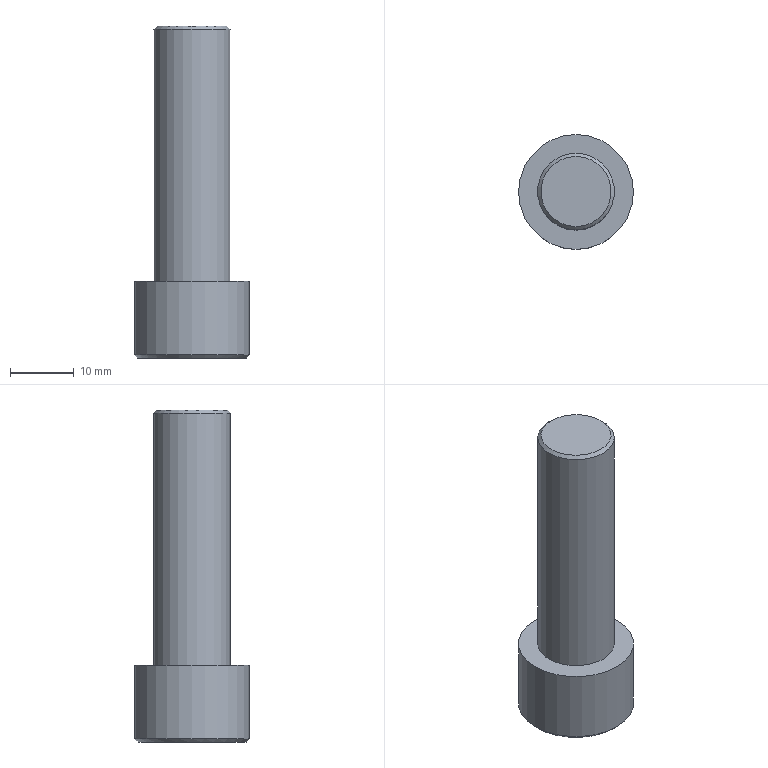Part | STEP file | 1_id1798_x_t | 1 solid | 21 faces | box 18 x 18 x 52 mm | volume 7011 mm3 | plane 15 | cone 4 | cylinder 2 | commonest cylinder face diameters 12 x1 18 x1
STEP:
#1=CARTESIAN_POINT('',(2147.435,399.726,-28.5));
#2=VERTEX_POINT('',#1);
#3=CARTESIAN_POINT('',(2147.435,405.5,-27.5));
#4=VERTEX_POINT('',#3);
#5=CARTESIAN_POINT('',(2147.435,402.613,-28.));
#6=DIRECTION('',(0.,0.9853,0.1707));
#7=VECTOR('',#6,1.);
#8=LINE('',#5,#7);
#9=EDGE_CURVE('',#2,#4,#8,.T.);
#10=ORIENTED_EDGE('',*,*,#9,.T.);
#11=CARTESIAN_POINT('',(2147.435,411.274,-28.5));
#12=VERTEX_POINT('',#11);
#13=CARTESIAN_POINT('',(2147.435,408.387,-28.));
#14=DIRECTION('',(0.,0.9853,-0.1707));
#15=VECTOR('',#14,1.);
#16=LINE('',#13,#15);
#17=EDGE_CURVE('',#4,#12,#16,.T.);
#18=ORIENTED_EDGE('',*,*,#17,.T.);
#19=CARTESIAN_POINT('',(2150.322,410.5,-28.5));
#20=VERTEX_POINT('',#19);
#21=CARTESIAN_POINT('',(2147.435,405.5,-28.5));
#22=DIRECTION('',(0.,0.,-1.));
#23=DIRECTION('',(0.,1.,0.));
#24=AXIS2_PLACEMENT_3D('',#21,#22,#23);
#25=CIRCLE('',#24,5.774);
#26=EDGE_CURVE('',#12,#20,#25,.T.);
#27=ORIENTED_EDGE('',*,*,#26,.T.);
#28=CARTESIAN_POINT('',(2153.209,405.5,-28.5));
#29=VERTEX_POINT('',#28);
#30=CARTESIAN_POINT('',(2147.435,405.5,-28.5));
#31=DIRECTION('',(0.,0.,-1.));
#32=DIRECTION('',(0.,1.,0.));
#33=AXIS2_PLACEMENT_3D('',#30,#31,#32);
#34=CIRCLE('',#33,5.774);
#35=EDGE_CURVE('',#20,#29,#34,.T.);
#36=ORIENTED_EDGE('',*,*,#35,.T.);
#37=CARTESIAN_POINT('',(2150.322,400.5,-28.5));
#38=VERTEX_POINT('',#37);
#39=CARTESIAN_POINT('',(2147.435,405.5,-28.5));
#40=DIRECTION('',(0.,0.,-1.));
#41=DIRECTION('',(0.,1.,0.));
#42=AXIS2_PLACEMENT_3D('',#39,#40,#41);
#43=CIRCLE('',#42,5.774);
#44=EDGE_CURVE('',#29,#38,#43,.T.);
#45=ORIENTED_EDGE('',*,*,#44,.T.);
#46=CARTESIAN_POINT('',(2147.435,405.5,-28.5));
#47=DIRECTION('',(0.,0.,-1.));
#48=DIRECTION('',(0.,1.,0.));
#49=AXIS2_PLACEMENT_3D('',#46,#47,#48);
#50=CIRCLE('',#49,5.774);
#51=EDGE_CURVE('',#38,#2,#50,.T.);
#52=ORIENTED_EDGE('',*,*,#51,.T.);
#53=EDGE_LOOP('',(#10,#18,#27,#36,#45,#52));
#54=FACE_OUTER_BOUND('',#53,.T.);
#55=CARTESIAN_POINT('',(2147.435,405.5,-28.));
#56=DIRECTION('',(0.,0.,-1.));
#57=DIRECTION('',(0.,-1.,0.));
#58=AXIS2_PLACEMENT_3D('',#55,#56,#57);
#59=CONICAL_SURFACE('',#58,2.887,80.174);
#60=ADVANCED_FACE('',(#54),#59,.F.);
#61=CARTESIAN_POINT('',(2147.435,399.5,17.));
#62=VERTEX_POINT('',#61);
#63=CARTESIAN_POINT('',(2147.435,405.5,17.));
#64=DIRECTION('',(0.,0.,1.));
#65=DIRECTION('',(0.,-1.,0.));
#66=AXIS2_PLACEMENT_3D('',#63,#64,#65);
#67=CIRCLE('',#66,6.);
#68=EDGE_CURVE('',#62,#62,#67,.T.);
#69=ORIENTED_EDGE('',*,*,#68,.T.);
#70=EDGE_LOOP('',(#69));
#71=FACE_BOUND('',#70,.T.);
#72=CARTESIAN_POINT('',(2147.435,400.,17.5));
#73=VERTEX_POINT('',#72);
#74=CARTESIAN_POINT('',(2147.435,405.5,17.5));
#75=DIRECTION('',(0.,0.,-1.));
#76=DIRECTION('',(0.,-1.,0.));
#77=AXIS2_PLACEMENT_3D('',#74,#75,#76);
#78=CIRCLE('',#77,5.5);
#79=EDGE_CURVE('',#73,#73,#78,.T.);
#80=ORIENTED_EDGE('',*,*,#79,.T.);
#81=EDGE_LOOP('',(#80));
#82=FACE_BOUND('',#81,.T.);
#83=CARTESIAN_POINT('',(2147.435,405.5,17.5));
#84=DIRECTION('',(0.,0.,-1.));
#85=DIRECTION('',(0.,1.,0.));
#86=AXIS2_PLACEMENT_3D('',#83,#84,#85);
#87=CONICAL_SURFACE('',#86,5.5,45.);
#88=ADVANCED_FACE('',(#71,#82),#87,.T.);
#89=ORIENTED_EDGE('',*,*,#68,.F.);
#90=EDGE_LOOP('',(#89));
#91=FACE_BOUND('',#90,.T.);
#92=CARTESIAN_POINT('',(2147.435,411.5,-22.5));
#93=VERTEX_POINT('',#92);
#94=CARTESIAN_POINT('',(2147.435,405.5,-22.5));
#95=DIRECTION('',(0.,0.,-1.));
#96=DIRECTION('',(0.,1.,0.));
#97=AXIS2_PLACEMENT_3D('',#94,#95,#96);
#98=CIRCLE('',#97,6.);
#99=EDGE_CURVE('',#93,#93,#98,.T.);
#100=ORIENTED_EDGE('',*,*,#99,.F.);
#101=EDGE_LOOP('',(#100));
#102=FACE_BOUND('',#101,.T.);
#103=CARTESIAN_POINT('',(2147.435,405.5,-2.5));
#104=DIRECTION('',(0.,0.,1.));
#105=DIRECTION('',(0.,-1.,0.));
#106=AXIS2_PLACEMENT_3D('',#103,#104,#105);
#107=CYLINDRICAL_SURFACE('',#106,6.);
#108=ADVANCED_FACE('',(#91,#102),#107,.T.);
#109=ORIENTED_EDGE('',*,*,#79,.F.);
#110=EDGE_LOOP('',(#109));
#111=FACE_OUTER_BOUND('',#110,.T.);
#112=CARTESIAN_POINT('',(2147.435,405.5,17.5));
#113=DIRECTION('',(0.,0.,1.));
#114=DIRECTION('',(0.,-1.,0.));
#115=AXIS2_PLACEMENT_3D('',#112,#113,#114);
#116=PLANE('',#115);
#117=ADVANCED_FACE('',(#111),#116,.T.);
#118=CARTESIAN_POINT('',(2147.435,396.5,-34.));
#119=VERTEX_POINT('',#118);
#120=CARTESIAN_POINT('',(2147.435,405.5,-34.));
#121=DIRECTION('',(0.,0.,-1.));
#122=DIRECTION('',(0.,-1.,0.));
#123=AXIS2_PLACEMENT_3D('',#120,#121,#122);
#124=CIRCLE('',#123,9.);
#125=EDGE_CURVE('',#119,#119,#124,.T.);
#126=ORIENTED_EDGE('',*,*,#125,.T.);
#127=EDGE_LOOP('',(#126));
#128=FACE_BOUND('',#127,.T.);
#129=CARTESIAN_POINT('',(2147.435,397.,-34.5));
#130=VERTEX_POINT('',#129);
#131=CARTESIAN_POINT('',(2147.435,405.5,-34.5));
#132=DIRECTION('',(0.,0.,1.));
#133=DIRECTION('',(0.,-1.,0.));
#134=AXIS2_PLACEMENT_3D('',#131,#132,#133);
#135=CIRCLE('',#134,8.5);
#136=EDGE_CURVE('',#130,#130,#135,.T.);
#137=ORIENTED_EDGE('',*,*,#136,.T.);
#138=EDGE_LOOP('',(#137));
#139=FACE_BOUND('',#138,.T.);
#140=CARTESIAN_POINT('',(2147.435,405.5,-34.5));
#141=DIRECTION('',(0.,0.,1.));
#142=DIRECTION('',(0.,1.,0.));
#143=AXIS2_PLACEMENT_3D('',#140,#141,#142);
#144=CONICAL_SURFACE('',#143,8.5,45.);
#145=ADVANCED_FACE('',(#128,#139),#144,.T.);
#146=CARTESIAN_POINT('',(2147.435,414.5,-22.5));
#147=VERTEX_POINT('',#146);
#148=CARTESIAN_POINT('',(2147.435,405.5,-22.5));
#149=DIRECTION('',(0.,0.,1.));
#150=DIRECTION('',(0.,1.,0.));
#151=AXIS2_PLACEMENT_3D('',#148,#149,#150);
#152=CIRCLE('',#151,9.);
#153=EDGE_CURVE('',#147,#147,#152,.T.);
#154=ORIENTED_EDGE('',*,*,#153,.F.);
#155=EDGE_LOOP('',(#154));
#156=FACE_BOUND('',#155,.T.);
#157=ORIENTED_EDGE('',*,*,#125,.F.);
#158=EDGE_LOOP('',(#157));
#159=FACE_BOUND('',#158,.T.);
#160=CARTESIAN_POINT('',(2147.435,405.5,-28.5));
#161=DIRECTION('',(0.,0.,1.));
#162=DIRECTION('',(0.,-1.,0.));
#163=AXIS2_PLACEMENT_3D('',#160,#161,#162);
#164=CYLINDRICAL_SURFACE('',#163,9.);
#165=ADVANCED_FACE('',(#156,#159),#164,.T.);
#166=CARTESIAN_POINT('',(2153.209,405.5,-34.5));
#167=VERTEX_POINT('',#166);
#168=CARTESIAN_POINT('',(2150.322,410.5,-34.5));
#169=VERTEX_POINT('',#168);
#170=CARTESIAN_POINT('',(2151.765,408.,-34.5));
#171=DIRECTION('',(-0.5,0.866,0.));
#172=VECTOR('',#171,1.);
#173=LINE('',#170,#172);
#174=EDGE_CURVE('',#167,#169,#173,.T.);
#175=ORIENTED_EDGE('',*,*,#174,.T.);
#176=CARTESIAN_POINT('',(2144.548,410.5,-34.5));
#177=VERTEX_POINT('',#176);
#178=CARTESIAN_POINT('',(2147.435,410.5,-34.5));
#179=DIRECTION('',(-1.,0.,0.));
#180=VECTOR('',#179,1.);
#181=LINE('',#178,#180);
#182=EDGE_CURVE('',#169,#177,#181,.T.);
#183=ORIENTED_EDGE('',*,*,#182,.T.);
#184=CARTESIAN_POINT('',(2141.662,405.5,-34.5));
#185=VERTEX_POINT('',#184);
#186=CARTESIAN_POINT('',(2143.105,408.,-34.5));
#187=DIRECTION('',(-0.5,-0.866,0.));
#188=VECTOR('',#187,1.);
#189=LINE('',#186,#188);
#190=EDGE_CURVE('',#177,#185,#189,.T.);
#191=ORIENTED_EDGE('',*,*,#190,.T.);
#192=CARTESIAN_POINT('',(2144.548,400.5,-34.5));
#193=VERTEX_POINT('',#192);
#194=CARTESIAN_POINT('',(2143.105,403.,-34.5));
#195=DIRECTION('',(0.5,-0.866,0.));
#196=VECTOR('',#195,1.);
#197=LINE('',#194,#196);
#198=EDGE_CURVE('',#185,#193,#197,.T.);
#199=ORIENTED_EDGE('',*,*,#198,.T.);
#200=CARTESIAN_POINT('',(2150.322,400.5,-34.5));
#201=VERTEX_POINT('',#200);
#202=CARTESIAN_POINT('',(2147.435,400.5,-34.5));
#203=DIRECTION('',(1.,0.,0.));
#204=VECTOR('',#203,1.);
#205=LINE('',#202,#204);
#206=EDGE_CURVE('',#193,#201,#205,.T.);
#207=ORIENTED_EDGE('',*,*,#206,.T.);
#208=CARTESIAN_POINT('',(2151.765,403.,-34.5));
#209=DIRECTION('',(0.5,0.866,0.));
#210=VECTOR('',#209,1.);
#211=LINE('',#208,#210);
#212=EDGE_CURVE('',#201,#167,#211,.T.);
#213=ORIENTED_EDGE('',*,*,#212,.T.);
#214=EDGE_LOOP('',(#175,#183,#191,#199,#207,#213));
#215=FACE_BOUND('',#214,.T.);
#216=ORIENTED_EDGE('',*,*,#136,.F.);
#217=EDGE_LOOP('',(#216));
#218=FACE_BOUND('',#217,.T.);
#219=CARTESIAN_POINT('',(2147.435,405.5,-34.5));
#220=DIRECTION('',(0.,0.,-1.));
#221=DIRECTION('',(0.,1.,0.));
#222=AXIS2_PLACEMENT_3D('',#219,#220,#221);
#223=PLANE('',#222);
#224=ADVANCED_FACE('',(#215,#218),#223,.T.);
#225=CARTESIAN_POINT('',(2151.765,408.,-28.5));
#226=DIRECTION('',(-0.5,0.866,0.));
#227=VECTOR('',#226,1.);
#228=LINE('',#225,#227);
#229=EDGE_CURVE('',#29,#20,#228,.T.);
#230=ORIENTED_EDGE('',*,*,#229,.F.);
#231=ORIENTED_EDGE('',*,*,#35,.F.);
#232=EDGE_LOOP('',(#230,#231));
#233=FACE_OUTER_BOUND('',#232,.T.);
#234=CARTESIAN_POINT('',(2147.435,405.5,-28.5));
#235=DIRECTION('',(0.,0.,-1.));
#236=DIRECTION('',(0.,1.,0.));
#237=AXIS2_PLACEMENT_3D('',#234,#235,#236);
#238=PLANE('',#237);
#239=ADVANCED_FACE('',(#233),#238,.F.);
#240=CARTESIAN_POINT('',(2144.548,410.5,-28.5));
#241=VERTEX_POINT('',#240);
#242=CARTESIAN_POINT('',(2147.435,410.5,-28.5));
#243=DIRECTION('',(-1.,0.,0.));
#244=VECTOR('',#243,1.);
#245=LINE('',#242,#244);
#246=EDGE_CURVE('',#20,#241,#245,.T.);
#247=ORIENTED_EDGE('',*,*,#246,.F.);
#248=ORIENTED_EDGE('',*,*,#26,.F.);
#249=CARTESIAN_POINT('',(2147.435,405.5,-28.5));
#250=DIRECTION('',(0.,0.,-1.));
#251=DIRECTION('',(0.,1.,0.));
#252=AXIS2_PLACEMENT_3D('',#249,#250,#251);
#253=CIRCLE('',#252,5.774);
#254=EDGE_CURVE('',#241,#12,#253,.T.);
#255=ORIENTED_EDGE('',*,*,#254,.F.);
#256=EDGE_LOOP('',(#247,#248,#255));
#257=FACE_OUTER_BOUND('',#256,.T.);
#258=CARTESIAN_POINT('',(2147.435,405.5,-28.5));
#259=DIRECTION('',(0.,0.,-1.));
#260=DIRECTION('',(0.,1.,0.));
#261=AXIS2_PLACEMENT_3D('',#258,#259,#260);
#262=PLANE('',#261);
#263=ADVANCED_FACE('',(#257),#262,.F.);
#264=CARTESIAN_POINT('',(2141.662,405.5,-28.5));
#265=VERTEX_POINT('',#264);
#266=CARTESIAN_POINT('',(2143.105,408.,-28.5));
#267=DIRECTION('',(-0.5,-0.866,0.));
#268=VECTOR('',#267,1.);
#269=LINE('',#266,#268);
#270=EDGE_CURVE('',#241,#265,#269,.T.);
#271=ORIENTED_EDGE('',*,*,#270,.F.);
#272=CARTESIAN_POINT('',(2147.435,405.5,-28.5));
#273=DIRECTION('',(0.,0.,-1.));
#274=DIRECTION('',(0.,1.,0.));
#275=AXIS2_PLACEMENT_3D('',#272,#273,#274);
#276=CIRCLE('',#275,5.774);
#277=EDGE_CURVE('',#265,#241,#276,.T.);
#278=ORIENTED_EDGE('',*,*,#277,.F.);
#279=EDGE_LOOP('',(#271,#278));
#280=FACE_OUTER_BOUND('',#279,.T.);
#281=CARTESIAN_POINT('',(2147.435,405.5,-28.5));
#282=DIRECTION('',(0.,0.,-1.));
#283=DIRECTION('',(0.,1.,0.));
#284=AXIS2_PLACEMENT_3D('',#281,#282,#283);
#285=PLANE('',#284);
#286=ADVANCED_FACE('',(#280),#285,.F.);
#287=CARTESIAN_POINT('',(2144.548,400.5,-28.5));
#288=VERTEX_POINT('',#287);
#289=CARTESIAN_POINT('',(2143.105,403.,-28.5));
#290=DIRECTION('',(0.5,-0.866,0.));
#291=VECTOR('',#290,1.);
#292=LINE('',#289,#291);
#293=EDGE_CURVE('',#265,#288,#292,.T.);
#294=ORIENTED_EDGE('',*,*,#293,.F.);
#295=CARTESIAN_POINT('',(2147.435,405.5,-28.5));
#296=DIRECTION('',(0.,0.,-1.));
#297=DIRECTION('',(0.,1.,0.));
#298=AXIS2_PLACEMENT_3D('',#295,#296,#297);
#299=CIRCLE('',#298,5.774);
#300=EDGE_CURVE('',#288,#265,#299,.T.);
#301=ORIENTED_EDGE('',*,*,#300,.F.);
#302=EDGE_LOOP('',(#294,#301));
#303=FACE_OUTER_BOUND('',#302,.T.);
#304=CARTESIAN_POINT('',(2147.435,405.5,-28.5));
#305=DIRECTION('',(0.,0.,-1.));
#306=DIRECTION('',(0.,1.,0.));
#307=AXIS2_PLACEMENT_3D('',#304,#305,#306);
#308=PLANE('',#307);
#309=ADVANCED_FACE('',(#303),#308,.F.);
#310=CARTESIAN_POINT('',(2147.435,400.5,-28.5));
#311=DIRECTION('',(1.,0.,0.));
#312=VECTOR('',#311,1.);
#313=LINE('',#310,#312);
#314=EDGE_CURVE('',#288,#38,#313,.T.);
#315=ORIENTED_EDGE('',*,*,#314,.F.);
#316=CARTESIAN_POINT('',(2147.435,405.5,-28.5));
#317=DIRECTION('',(0.,0.,-1.));
#318=DIRECTION('',(0.,1.,0.));
#319=AXIS2_PLACEMENT_3D('',#316,#317,#318);
#320=CIRCLE('',#319,5.774);
#321=EDGE_CURVE('',#2,#288,#320,.T.);
#322=ORIENTED_EDGE('',*,*,#321,.F.);
#323=ORIENTED_EDGE('',*,*,#51,.F.);
#324=EDGE_LOOP('',(#315,#322,#323));
#325=FACE_OUTER_BOUND('',#324,.T.);
#326=CARTESIAN_POINT('',(2147.435,405.5,-28.5));
#327=DIRECTION('',(0.,0.,-1.));
#328=DIRECTION('',(0.,1.,0.));
#329=AXIS2_PLACEMENT_3D('',#326,#327,#328);
#330=PLANE('',#329);
#331=ADVANCED_FACE('',(#325),#330,.F.);
#332=CARTESIAN_POINT('',(2151.765,403.,-28.5));
#333=DIRECTION('',(0.5,0.866,0.));
#334=VECTOR('',#333,1.);
#335=LINE('',#332,#334);
#336=EDGE_CURVE('',#38,#29,#335,.T.);
#337=ORIENTED_EDGE('',*,*,#336,.F.);
#338=ORIENTED_EDGE('',*,*,#44,.F.);
#339=EDGE_LOOP('',(#337,#338));
#340=FACE_OUTER_BOUND('',#339,.T.);
#341=CARTESIAN_POINT('',(2147.435,405.5,-28.5));
#342=DIRECTION('',(0.,0.,-1.));
#343=DIRECTION('',(0.,1.,0.));
#344=AXIS2_PLACEMENT_3D('',#341,#342,#343);
#345=PLANE('',#344);
#346=ADVANCED_FACE('',(#340),#345,.F.);
#347=ORIENTED_EDGE('',*,*,#9,.F.);
#348=ORIENTED_EDGE('',*,*,#321,.T.);
#349=ORIENTED_EDGE('',*,*,#300,.T.);
#350=ORIENTED_EDGE('',*,*,#277,.T.);
#351=ORIENTED_EDGE('',*,*,#254,.T.);
#352=ORIENTED_EDGE('',*,*,#17,.F.);
#353=EDGE_LOOP('',(#347,#348,#349,#350,#351,#352));
#354=FACE_OUTER_BOUND('',#353,.T.);
#355=CARTESIAN_POINT('',(2147.435,405.5,-28.));
#356=DIRECTION('',(0.,0.,-1.));
#357=DIRECTION('',(0.,-1.,0.));
#358=AXIS2_PLACEMENT_3D('',#355,#356,#357);
#359=CONICAL_SURFACE('',#358,2.887,80.174);
#360=ADVANCED_FACE('',(#354),#359,.F.);
#361=CARTESIAN_POINT('',(2153.209,405.5,-31.5));
#362=DIRECTION('',(0.,0.,-1.));
#363=VECTOR('',#362,1.);
#364=LINE('',#361,#363);
#365=EDGE_CURVE('',#29,#167,#364,.T.);
#366=ORIENTED_EDGE('',*,*,#365,.F.);
#367=ORIENTED_EDGE('',*,*,#229,.T.);
#368=CARTESIAN_POINT('',(2150.322,410.5,-31.5));
#369=DIRECTION('',(0.,0.,-1.));
#370=VECTOR('',#369,1.);
#371=LINE('',#368,#370);
#372=EDGE_CURVE('',#20,#169,#371,.T.);
#373=ORIENTED_EDGE('',*,*,#372,.T.);
#374=ORIENTED_EDGE('',*,*,#174,.F.);
#375=EDGE_LOOP('',(#366,#367,#373,#374));
#376=FACE_OUTER_BOUND('',#375,.T.);
#377=CARTESIAN_POINT('',(2151.765,408.,-31.5));
#378=DIRECTION('',(-0.866,-0.5,0.));
#379=DIRECTION('',(0.,0.,-1.));
#380=AXIS2_PLACEMENT_3D('',#377,#378,#379);
#381=PLANE('',#380);
#382=ADVANCED_FACE('',(#376),#381,.T.);
#383=CARTESIAN_POINT('',(2150.322,400.5,-31.5));
#384=DIRECTION('',(0.,0.,-1.));
#385=VECTOR('',#384,1.);
#386=LINE('',#383,#385);
#387=EDGE_CURVE('',#38,#201,#386,.T.);
#388=ORIENTED_EDGE('',*,*,#387,.F.);
#389=ORIENTED_EDGE('',*,*,#336,.T.);
#390=ORIENTED_EDGE('',*,*,#365,.T.);
#391=ORIENTED_EDGE('',*,*,#212,.F.);
#392=EDGE_LOOP('',(#388,#389,#390,#391));
#393=FACE_OUTER_BOUND('',#392,.T.);
#394=CARTESIAN_POINT('',(2151.765,403.,-31.5));
#395=DIRECTION('',(-0.866,0.5,0.));
#396=DIRECTION('',(0.,0.,1.));
#397=AXIS2_PLACEMENT_3D('',#394,#395,#396);
#398=PLANE('',#397);
#399=ADVANCED_FACE('',(#393),#398,.T.);
#400=CARTESIAN_POINT('',(2144.548,400.5,-31.5));
#401=DIRECTION('',(0.,0.,-1.));
#402=VECTOR('',#401,1.);
#403=LINE('',#400,#402);
#404=EDGE_CURVE('',#288,#193,#403,.T.);
#405=ORIENTED_EDGE('',*,*,#404,.F.);
#406=ORIENTED_EDGE('',*,*,#314,.T.);
#407=ORIENTED_EDGE('',*,*,#387,.T.);
#408=ORIENTED_EDGE('',*,*,#206,.F.);
#409=EDGE_LOOP('',(#405,#406,#407,#408));
#410=FACE_OUTER_BOUND('',#409,.T.);
#411=CARTESIAN_POINT('',(2147.435,400.5,-31.5));
#412=DIRECTION('',(0.,1.,0.));
#413=DIRECTION('',(0.,0.,1.));
#414=AXIS2_PLACEMENT_3D('',#411,#412,#413);
#415=PLANE('',#414);
#416=ADVANCED_FACE('',(#410),#415,.T.);
#417=CARTESIAN_POINT('',(2141.662,405.5,-31.5));
#418=DIRECTION('',(0.,0.,-1.));
#419=VECTOR('',#418,1.);
#420=LINE('',#417,#419);
#421=EDGE_CURVE('',#265,#185,#420,.T.);
#422=ORIENTED_EDGE('',*,*,#421,.F.);
#423=ORIENTED_EDGE('',*,*,#293,.T.);
#424=ORIENTED_EDGE('',*,*,#404,.T.);
#425=ORIENTED_EDGE('',*,*,#198,.F.);
#426=EDGE_LOOP('',(#422,#423,#424,#425));
#427=FACE_OUTER_BOUND('',#426,.T.);
#428=CARTESIAN_POINT('',(2143.105,403.,-31.5));
#429=DIRECTION('',(0.866,0.5,0.));
#430=DIRECTION('',(0.,0.,1.));
#431=AXIS2_PLACEMENT_3D('',#428,#429,#430);
#432=PLANE('',#431);
#433=ADVANCED_FACE('',(#427),#432,.T.);
#434=CARTESIAN_POINT('',(2144.548,410.5,-31.5));
#435=DIRECTION('',(0.,0.,-1.));
#436=VECTOR('',#435,1.);
#437=LINE('',#434,#436);
#438=EDGE_CURVE('',#241,#177,#437,.T.);
#439=ORIENTED_EDGE('',*,*,#438,.F.);
#440=ORIENTED_EDGE('',*,*,#270,.T.);
#441=ORIENTED_EDGE('',*,*,#421,.T.);
#442=ORIENTED_EDGE('',*,*,#190,.F.);
#443=EDGE_LOOP('',(#439,#440,#441,#442));
#444=FACE_OUTER_BOUND('',#443,.T.);
#445=CARTESIAN_POINT('',(2143.105,408.,-31.5));
#446=DIRECTION('',(0.866,-0.5,0.));
#447=DIRECTION('',(0.,0.,-1.));
#448=AXIS2_PLACEMENT_3D('',#445,#446,#447);
#449=PLANE('',#448);
#450=ADVANCED_FACE('',(#444),#449,.T.);
#451=ORIENTED_EDGE('',*,*,#372,.F.);
#452=ORIENTED_EDGE('',*,*,#246,.T.);
#453=ORIENTED_EDGE('',*,*,#438,.T.);
#454=ORIENTED_EDGE('',*,*,#182,.F.);
#455=EDGE_LOOP('',(#451,#452,#453,#454));
#456=FACE_OUTER_BOUND('',#455,.T.);
#457=CARTESIAN_POINT('',(2147.435,410.5,-31.5));
#458=DIRECTION('',(0.,-1.,0.));
#459=DIRECTION('',(0.,0.,-1.));
#460=AXIS2_PLACEMENT_3D('',#457,#458,#459);
#461=PLANE('',#460);
#462=ADVANCED_FACE('',(#456),#461,.T.);
#463=ORIENTED_EDGE('',*,*,#99,.T.);
#464=EDGE_LOOP('',(#463));
#465=FACE_BOUND('',#464,.T.);
#466=ORIENTED_EDGE('',*,*,#153,.T.);
#467=EDGE_LOOP('',(#466));
#468=FACE_BOUND('',#467,.T.);
#469=CARTESIAN_POINT('',(2147.435,405.5,-22.5));
#470=DIRECTION('',(0.,0.,1.));
#471=DIRECTION('',(0.,-1.,0.));
#472=AXIS2_PLACEMENT_3D('',#469,#470,#471);
#473=PLANE('',#472);
#474=ADVANCED_FACE('',(#465,#468),#473,.T.);
#475=CLOSED_SHELL('',(#60,#88,#108,#117,#145,#165,#224,#239,#263,#286,#309,#331,#346,#360,#382,#399,#416,#433,#450,#462,#474));
#476=MANIFOLD_SOLID_BREP('',#475);
#477=(LENGTH_UNIT()NAMED_UNIT(*)SI_UNIT(.MILLI.,.METRE.));
#478=UNCERTAINTY_MEASURE_WITH_UNIT(LENGTH_MEASURE(0.00002),#477,'','');
#479=(NAMED_UNIT(*)PLANE_ANGLE_UNIT()SI_UNIT($,.RADIAN.));
#480=PLANE_ANGLE_MEASURE_WITH_UNIT(PLANE_ANGLE_MEASURE(0.01745),#479);
#481=DIMENSIONAL_EXPONENTS(0.,0.,0.,0.,0.,0.,0.);
#482=(CONVERSION_BASED_UNIT('DEGREE',#480)NAMED_UNIT(#481)PLANE_ANGLE_UNIT());
#483=(NAMED_UNIT(*)SI_UNIT($,.STERADIAN.)SOLID_ANGLE_UNIT());
#484=(GEOMETRIC_REPRESENTATION_CONTEXT(3)GLOBAL_UNCERTAINTY_ASSIGNED_CONTEXT((#478))GLOBAL_UNIT_ASSIGNED_CONTEXT((#477,#482,#483))REPRESENTATION_CONTEXT('',''));
#485=ADVANCED_BREP_SHAPE_REPRESENTATION('',(#476),#484);